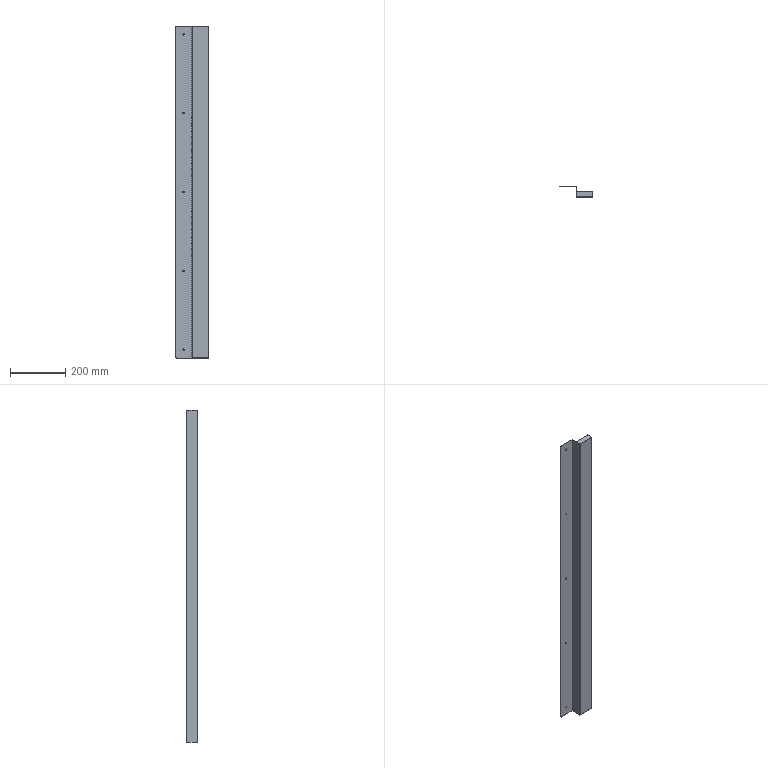Part | SolidWorks | features ICE 4, ExtruThin 1, Fillet 1, FlatPattern 1, FlattenBends 1, ProcessBends 1, SheetMetal 1 | 1 solid | 62 faces | box 120 x 40 x 1200 mm | volume 129437 mm3 | plane 40 | cylinder 22 | commonest cylinder face diameters 5.5 x10 0.6 x5 1.8 x5 10 x2